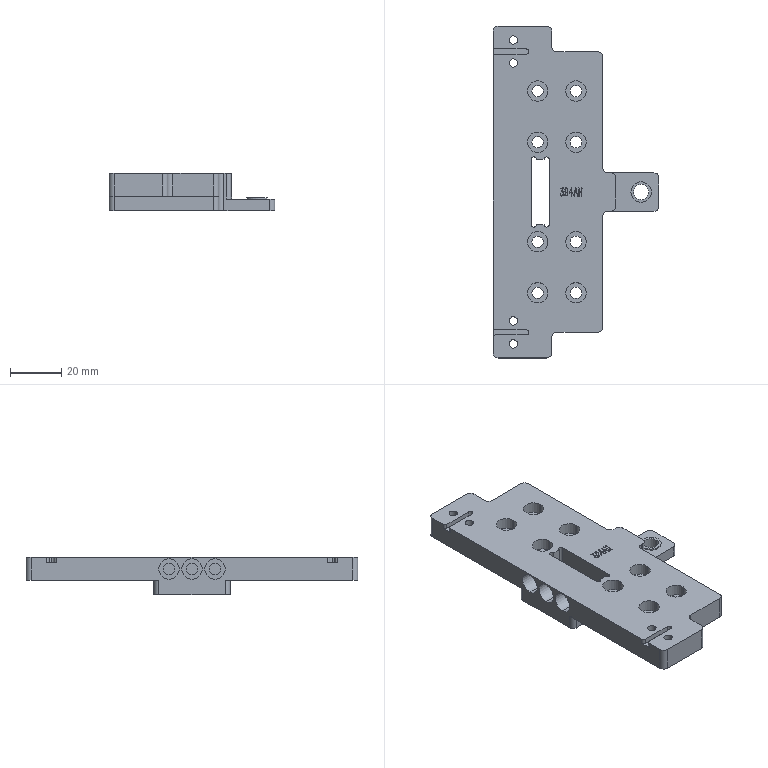NC program | NX | posted with a generic post | part box 65 x 130 x 14.5 mm
Lines 2189 to 4086 of 11202, first 1613 of 1886 lines:
(ZLEVEL_PROFILE_COPY_1_COPY_COPY_1 , TOOL : D10JING)
N4328 T14 M6
N4330 G54
N4332 G17 G0 G90 X64.645 Y-39.348 B0. C0. S9500 M3
N4334 G43 Z30. H14
N4336 Z-13.5
N4338 G94 G1 Z-14.5 F1000.
N4340 X63.866 Y-38.
N4342 G3 X63. Y-37.5 R1.
N4344 G1 X-63. F1200.
N4346 G2 X-70. Y-30.5 R7.
N4348 G1 Y-11.5
N4350 G2 X-63. Y-4.5 R7.
N4352 G1 X-60.
N4354 Y8.5
N4356 G2 X-53. Y15.5 R7.
N4358 G1 X-12.5
N4360 Y30.5
N4362 G2 X-5.5 Y37.5 R7.
N4364 G1 X5.5
N4366 G2 X12.5 Y30.5 R7.
N4368 G1 Y15.5
N4370 X53.
N4372 G2 X60. Y8.5 R7.
N4374 G1 Y-4.5
N4376 X63.
N4378 G2 X70. Y-11.5 R7.
N4380 G1 Y-30.5
N4382 G2 X63. Y-37.5 R7.
N4384 G3 X62.134 Y-38. R1.
N4386 G1 X61.268 Y-39.5
N4388 Z-13.5
N4390 G0 Z30.
N4392 M5
(FLOOR_WALL , TOOL : D4)
N4394 T11 M6
N4396 G54
N4398 G17 G0 G90 X-7.417 Y24.39 B0. C0. S9500 M3
N4400 G43 Z30. H11
N4402 Z-8.
N4404 G94 G1 Z-9.5 F1250.
N4406 X-6.2 Y25.093
N4408 G3 X-6. Y25.44 R0.4
N4410 G1 Y25.56
N4412 G2 X-4.32 Y29.664 R6.
N4414 G1 Y21.336
N4416 G3 X-2.64 Y20.112 R6.
N4418 G1 Y30.888
N4420 G2 X-0.96 Y31.423 R6.
N4422 G1 Y19.577
N4424 G3 X0. Y19.5 R6.
N4426 X0.72 Y19.543 R6.
N4428 G1 X0.719 Y31.457
N4430 G2 X2.399 Y30.999 R6.
N4432 G1 X2.4 Y20.001
N4434 G2 X2.2 Y19.654 R0.4
N4436 G1 X3.742 Y19.
N4438 Z-8.
N4440 G0 Z30.
N4442 X11. Y14.995
N4444 Z-8.5
N4446 G1 Z-10.
N4448 X9.846 Y16.993
N4450 G3 X9.5 Y17.193 R0.4
N4452 G1 X7.5
N4454 G3 X5.5 Y17.7 R4.2
N4456 G1 X-5.5
N4458 G3 X-7.5 Y17.193 R4.2
N4460 G1 X-9.5
N4462 Y19.151
N4464 X9.5
N4466 Y21.109
N4468 X4.378
N4470 G3 X5.703 Y23.068 R6.2
N4472 G1 X9.5
N4474 Y25.026
N4476 X6.182
N4478 G3 X6.02 Y26.984 R6.2
N4480 G1 X9.5
N4482 Y28.942
N4484 X5.157
N4486 G3 X3.046 Y30.9 R6.2
N4488 G1 X9.48
N4490 G2 X9.826 Y30.7 R0.4
N4492 G1 X11. Y28.667
N4494 Z-8.5
N4496 G0 Z30.
N4498 X4.378 Y21.109
N4500 Z-8.5
N4502 G1 Z-10.
N4504 G2 X-4.378 Y21.109 R6.2
N4506 G1 X-9.5
N4508 Y23.068
N4510 X-5.703
N4512 G2 X-6.182 Y25.026 R6.2
N4514 G1 X-9.5
N4516 Y26.984
N4518 X-6.02
N4520 G2 X-5.157 Y28.942 R6.2
N4522 G1 X-9.5
N4524 Y30.5
N4526 G2 X-9.48 Y30.9 R4.
N4528 G1 X-3.046
N4530 Z-8.5
N4532 G0 Z30.
N4534 X10.209 Y33.341
N4536 Z-8.5
N4538 G1 Z-10.
N4540 X9.077 Y32.658
N4542 G3 X8.731 Y32.858 R0.4
N4544 G1 X-8.731
N4546 G3 X-9.077 Y32.658 R0.4
N4548 G1 X-10.209 Y33.341
N4550 Z-8.5
N4552 G0 Z30.
N4554 X-11. Y14.
N4556 Z-8.5
N4558 G1 Z-10.
N4560 X-9.711 Y13.67
N4562 G3 X-9.47 Y13.989 R0.4
N4564 G2 X-5.5 Y17.5 R4.
N4566 G1 X5.5
N4568 G2 X9.47 Y13.989 R4.
N4570 G3 X9.711 Y13.67 R0.4
N4572 G1 X11. Y14.
N4574 Z-8.5
N4576 G0 Z30.
N4578 X-1.744 Y33.
N4580 Z-8.5
N4582 G1 Z-10.
N4584 X-0.346 Y31.7
N4586 G3 X0. Y31.5 R0.4
N4588 G2 X6. Y25.5 R6.
N4590 X0. Y31.5 R-6.
N4592 G3 X0.346 Y31.7 R0.4
N4594 G1 X1.162 Y33.112
N4596 Z-8.5
N4598 G0 Z30.
(HOLE_MILLING , TOOL : D4)
N4600 X0. Y25.5
N4602 Z-9.
N4604 G3 X0.45 Y25.95 R0.45
N4606 X0. Y26.4 R0.45
N4608 X0. Y26.4 Z-9.4 I0. J-0.9
N4610 X0. Y26.4 Z-9.8 I0. J-0.9
N4612 X0. Y26.4 Z-10.2 I0. J-0.9
N4614 X0. Y26.4 Z-10.6 I0. J-0.9
N4616 X0. Y26.4 Z-11. I0. J-0.9
N4618 X0. Y26.4 Z-11.4 I0. J-0.9
N4620 X0. Y26.4 Z-11.8 I0. J-0.9
N4622 X0. Y26.4 Z-12.2 I0. J-0.9
N4624 X0. Y26.4 Z-12.6 I0. J-0.9
N4626 X0. Y26.4 Z-13. I0. J-0.9
N4628 X0. Y26.4 Z-13.4 I0. J-0.9
N4630 X0. Y26.4 Z-13.8 I0. J-0.9
N4632 X0. Y26.4 Z-14.2 I0. J-0.9
N4634 X0.9 Y25.5 Z-14.5 R-0.9
N4636 X0. Y26.4 R0.9
N4638 X0.9 Y25.5 R-0.9
N4640 X0.45 Y25.95 R0.45
N4642 X0. Y25.5 R0.45
N4644 G0 Z30.
(HOLE_MILLING_COPY , TOOL : D4)
N4646 X-39.5 Y0.
N4648 Z0.5
N4650 G3 X-38.5 Y1. R1.
N4652 X-39.5 Y2. R1.
N4654 X-39.5 Y2. Z0.1 I0. J-2.
N4656 X-39.5 Y2. Z-0.3 I0. J-2.
N4658 X-39.5 Y2. Z-0.7 I0. J-2.
N4660 X-39.5 Y2. Z-1.1 I0. J-2.
N4662 X-39.5 Y2. Z-1.5 I0. J-2.
N4664 X-39.5 Y2. Z-1.9 I0. J-2.
N4666 X-39.5 Y2. Z-2.3 I0. J-2.
N4668 X-39.5 Y2. Z-2.7 I0. J-2.
N4670 X-39.5 Y2. Z-3.1 I0. J-2.
N4672 X-39.5 Y2. Z-3.5 I0. J-2.
N4674 X-39.5 Y2. Z-3.9 I0. J-2.
N4676 X-39.5 Y2. Z-4.3 I0. J-2.
N4678 X-37.5 Y0. Z-4.6 R-2.
N4680 X-39.5 Y2. R2.
N4682 X-37.5 Y0. R-2.
N4684 X-38.5 Y1. R1.
N4686 X-39.5 Y0. R1.
N4688 G0 Z30.
N4690 Y-15.
N4692 Z0.5
N4694 G3 X-38.5 Y-14. R1.
N4696 X-39.5 Y-13. R1.
N4698 X-39.5 Y-13. Z0.1 I0. J-2.
N4700 X-39.5 Y-13. Z-0.3 I0. J-2.
N4702 X-39.5 Y-13. Z-0.7 I0. J-2.
N4704 X-39.5 Y-13. Z-1.1 I0. J-2.
N4706 X-39.5 Y-13. Z-1.5 I0. J-2.
N4708 X-39.5 Y-13. Z-1.9 I0. J-2.
N4710 X-39.5 Y-13. Z-2.3 I0. J-2.
N4712 X-39.5 Y-13. Z-2.7 I0. J-2.
N4714 X-39.5 Y-13. Z-3.1 I0. J-2.
N4716 X-39.5 Y-13. Z-3.5 I0. J-2.
N4718 X-39.5 Y-13. Z-3.9 I0. J-2.
N4720 X-39.5 Y-13. Z-4.3 I0. J-2.
N4722 X-37.5 Y-15. Z-4.6 R-2.
N4724 X-39.5 Y-13. R2.
N4726 X-37.5 Y-15. R-2.
N4728 X-38.5 Y-14. R1.
N4730 X-39.5 Y-15. R1.
N4732 G0 Z30.
N4734 X-19.5
N4736 Z0.5
N4738 G3 X-18.5 Y-14. R1.
N4740 X-19.5 Y-13. R1.
N4742 X-19.5 Y-13. Z0.1 I0. J-2.
N4744 X-19.5 Y-13. Z-0.3 I0. J-2.
N4746 X-19.5 Y-13. Z-0.7 I0. J-2.
N4748 X-19.5 Y-13. Z-1.1 I0. J-2.
N4750 X-19.5 Y-13. Z-1.5 I0. J-2.
N4752 X-19.5 Y-13. Z-1.9 I0. J-2.
N4754 X-19.5 Y-13. Z-2.3 I0. J-2.
N4756 X-19.5 Y-13. Z-2.7 I0. J-2.
N4758 X-19.5 Y-13. Z-3.1 I0. J-2.
N4760 X-19.5 Y-13. Z-3.5 I0. J-2.
N4762 X-19.5 Y-13. Z-3.9 I0. J-2.
N4764 X-19.5 Y-13. Z-4.3 I0. J-2.
N4766 X-17.5 Y-15. Z-4.6 R-2.
N4768 X-19.5 Y-13. R2.
N4770 X-17.5 Y-15. R-2.
N4772 X-18.5 Y-14. R1.
N4774 X-19.5 Y-15. R1.
N4776 G0 Z30.
N4778 Y0.
N4780 Z0.5
N4782 G3 X-18.5 Y1. R1.
N4784 X-19.5 Y2. R1.
N4786 X-19.5 Y2. Z0.1 I0. J-2.
N4788 X-19.5 Y2. Z-0.3 I0. J-2.
N4790 X-19.5 Y2. Z-0.7 I0. J-2.
N4792 X-19.5 Y2. Z-1.1 I0. J-2.
N4794 X-19.5 Y2. Z-1.5 I0. J-2.
N4796 X-19.5 Y2. Z-1.9 I0. J-2.
N4798 X-19.5 Y2. Z-2.3 I0. J-2.
N4800 X-19.5 Y2. Z-2.7 I0. J-2.
N4802 X-19.5 Y2. Z-3.1 I0. J-2.
N4804 X-19.5 Y2. Z-3.5 I0. J-2.
N4806 X-19.5 Y2. Z-3.9 I0. J-2.
N4808 X-19.5 Y2. Z-4.3 I0. J-2.
N4810 X-17.5 Y0. Z-4.6 R-2.
N4812 X-19.5 Y2. R2.
N4814 X-17.5 Y0. R-2.
N4816 X-18.5 Y1. R1.
N4818 X-19.5 Y0. R1.
N4820 G0 Z30.
N4822 X19.5
N4824 Z0.5
N4826 G3 X20.5 Y1. R1.
N4828 X19.5 Y2. R1.
N4830 X19.5 Y2. Z0.1 I0. J-2.
N4832 X19.5 Y2. Z-0.3 I0. J-2.
N4834 X19.5 Y2. Z-0.7 I0. J-2.
N4836 X19.5 Y2. Z-1.1 I0. J-2.
N4838 X19.5 Y2. Z-1.5 I0. J-2.
N4840 X19.5 Y2. Z-1.9 I0. J-2.
N4842 X19.5 Y2. Z-2.3 I0. J-2.
N4844 X19.5 Y2. Z-2.7 I0. J-2.
N4846 X19.5 Y2. Z-3.1 I0. J-2.
N4848 X19.5 Y2. Z-3.5 I0. J-2.
N4850 X19.5 Y2. Z-3.9 I0. J-2.
N4852 X19.5 Y2. Z-4.3 I0. J-2.
N4854 X21.5 Y0. Z-4.6 R-2.
N4856 X19.5 Y2. R2.
N4858 X21.5 Y0. R-2.
N4860 X20.5 Y1. R1.
N4862 X19.5 Y0. R1.
N4864 G0 Z30.
N4866 Y-15.
N4868 Z0.5
N4870 G3 X20.5 Y-14. R1.
N4872 X19.5 Y-13. R1.
N4874 X19.5 Y-13. Z0.1 I0. J-2.
N4876 X19.5 Y-13. Z-0.3 I0. J-2.
N4878 X19.5 Y-13. Z-0.7 I0. J-2.
N4880 X19.5 Y-13. Z-1.1 I0. J-2.
N4882 X19.5 Y-13. Z-1.5 I0. J-2.
N4884 X19.5 Y-13. Z-1.9 I0. J-2.
N4886 X19.5 Y-13. Z-2.3 I0. J-2.
N4888 X19.5 Y-13. Z-2.7 I0. J-2.
N4890 X19.5 Y-13. Z-3.1 I0. J-2.
N4892 X19.5 Y-13. Z-3.5 I0. J-2.
N4894 X19.5 Y-13. Z-3.9 I0. J-2.
N4896 X19.5 Y-13. Z-4.3 I0. J-2.
N4898 X21.5 Y-15. Z-4.6 R-2.
N4900 X19.5 Y-13. R2.
N4902 X21.5 Y-15. R-2.
N4904 X20.5 Y-14. R1.
N4906 X19.5 Y-15. R1.
N4908 G0 Z30.
N4910 X39.5
N4912 Z0.5
N4914 G3 X40.5 Y-14. R1.
N4916 X39.5 Y-13. R1.
N4918 X39.5 Y-13. Z0.1 I0. J-2.
N4920 X39.5 Y-13. Z-0.3 I0. J-2.
N4922 X39.5 Y-13. Z-0.7 I0. J-2.
N4924 X39.5 Y-13. Z-1.1 I0. J-2.
N4926 X39.5 Y-13. Z-1.5 I0. J-2.
N4928 X39.5 Y-13. Z-1.9 I0. J-2.
N4930 X39.5 Y-13. Z-2.3 I0. J-2.
N4932 X39.5 Y-13. Z-2.7 I0. J-2.
N4934 X39.5 Y-13. Z-3.1 I0. J-2.
N4936 X39.5 Y-13. Z-3.5 I0. J-2.
N4938 X39.5 Y-13. Z-3.9 I0. J-2.
N4940 X39.5 Y-13. Z-4.3 I0. J-2.
N4942 X41.5 Y-15. Z-4.6 R-2.
N4944 X39.5 Y-13. R2.
N4946 X41.5 Y-15. R-2.
N4948 X40.5 Y-14. R1.
N4950 X39.5 Y-15. R1.
N4952 G0 Z30.
N4954 Y0.
N4956 Z0.5
N4958 G3 X40.5 Y1. R1.
N4960 X39.5 Y2. R1.
N4962 X39.5 Y2. Z0.1 I0. J-2.
N4964 X39.5 Y2. Z-0.3 I0. J-2.
N4966 X39.5 Y2. Z-0.7 I0. J-2.
N4968 X39.5 Y2. Z-1.1 I0. J-2.
N4970 X39.5 Y2. Z-1.5 I0. J-2.
N4972 X39.5 Y2. Z-1.9 I0. J-2.
N4974 X39.5 Y2. Z-2.3 I0. J-2.
N4976 X39.5 Y2. Z-2.7 I0. J-2.
N4978 X39.5 Y2. Z-3.1 I0. J-2.
N4980 X39.5 Y2. Z-3.5 I0. J-2.
N4982 X39.5 Y2. Z-3.9 I0. J-2.
N4984 X39.5 Y2. Z-4.3 I0. J-2.
N4986 X41.5 Y0. Z-4.6 R-2.
N4988 X39.5 Y2. R2.
N4990 X41.5 Y0. R-2.
N4992 X40.5 Y1. R1.
N4994 X39.5 Y0. R1.
N4996 G0 Z30.
(ZLEVEL_PROFILE , TOOL : D4)
N4998 X1.453 Y-15.4
N5000 Z1.5
N5002 G1 X10.65 Z1.018 F1000.
N5004 Y-12.6 Z0.871
N5006 X-10.653 Z-0.245
N5008 X-10.65 Y-12.637 Z-0.247
N5010 Y-15.363 Z-0.39
N5012 X-10.653 Y-15.4 Z-0.392
N5014 X10.65 F1800.
N5016 Y-12.6
N5018 X-10.653
N5020 X-10.65 Y-12.637
N5022 Y-15.363
N5024 X-10.653 Y-15.4
N5026 X-10.508 Z-0.394
N5028 X10.64 Z-0.764
N5030 X10.65 Y-15.265 Z-0.766
N5032 Y-14.251 Z-0.784
N5034 Y-12.6
N5036 X-10.653
N5038 X-10.65 Y-12.637
N5040 Y-15.363
N5042 X-10.653 Y-15.4
N5044 X-10.508 Z-0.786
N5046 X10.64 Z-1.155
N5048 X10.65 Y-15.265 Z-1.158
N5050 Y-14.251 Z-1.176
N5052 Y-12.6
N5054 X-10.653
N5056 X-10.65 Y-12.637
N5058 Y-15.363
N5060 X-10.653 Y-15.4
N5062 X-10.508 Z-1.178
N5064 X10.64 Z-1.547
N5066 X10.65 Y-15.265 Z-1.55
N5068 Y-14.251 Z-1.568
N5070 Y-12.6
N5072 X-10.653
N5074 X-10.65 Y-12.637
N5076 Y-15.363
N5078 X-10.653 Y-15.4
N5080 X-10.508 Z-1.57
N5082 X10.64 Z-1.939
N5084 X10.65 Y-15.265 Z-1.942
N5086 Y-14.251 Z-1.959
N5088 Y-12.6
N5090 X-10.653
N5092 X-10.65 Y-12.637
N5094 Y-15.363
N5096 X-10.653 Y-15.4
N5098 X-10.508 Z-1.962
N5100 X10.64 Z-2.331
N5102 X10.65 Y-15.265 Z-2.334
N5104 Y-14.251 Z-2.351
N5106 Y-12.6
N5108 X-10.653
N5110 X-10.65 Y-12.637
N5112 Y-15.363
N5114 X-10.653 Y-15.4
N5116 X-10.508 Z-2.354
N5118 X10.64 Z-2.723
N5120 X10.65 Y-15.265 Z-2.726
N5122 Y-14.251 Z-2.743
N5124 Y-12.6
N5126 X-10.653
N5128 X-10.65 Y-12.637
N5130 Y-15.363
N5132 X-10.653 Y-15.4
N5134 X-10.508 Z-2.746
N5136 X10.64 Z-3.115
N5138 X10.65 Y-15.265 Z-3.117
N5140 Y-14.251 Z-3.135
N5142 Y-12.6
N5144 X-10.653
N5146 X-10.65 Y-12.637
N5148 Y-15.363
N5150 X-10.653 Y-15.4
N5152 X-10.508 Z-3.138
N5154 X10.64 Z-3.507
N5156 X10.65 Y-15.265 Z-3.509
N5158 Y-14.251 Z-3.527
N5160 Y-12.6
N5162 X-10.652
N5164 X-10.65 Y-12.637
N5166 Y-15.363
N5168 X-10.652 Y-15.4
N5170 X-10.508 Z-3.53
N5172 X10.64 Z-3.899
N5174 X10.65 Y-15.265 Z-3.901
N5176 Y-14.251 Z-3.919
N5178 Y-12.6
N5180 X-10.652
N5182 X-10.65 Y-12.637
N5184 Y-15.363
N5186 X-10.652 Y-15.4
N5188 X-10.508 Z-3.921
N5190 X10.64 Z-4.291
N5192 X10.65 Y-15.265 Z-4.293
N5194 Y-14.251 Z-4.311
N5196 Y-12.6
N5198 X-10.652
N5200 X-10.65 Y-12.637
N5202 Y-15.363
N5204 X-10.652 Y-15.4
N5206 X-10.508 Z-4.313
N5208 X10.64 Z-4.682
N5210 X10.65 Y-15.265 Z-4.685
N5212 Y-14.251 Z-4.703
N5214 Y-12.6
N5216 X-10.652
N5218 X-10.65 Y-12.637
N5220 Y-15.363
N5222 X-10.652 Y-15.4
N5224 X-10.508 Z-4.705
N5226 X10.64 Z-5.074
N5228 X10.65 Y-15.265 Z-5.077
N5230 Y-14.251 Z-5.095
N5232 Y-12.6
N5234 X-10.652
N5236 X-10.65 Y-12.637
N5238 Y-15.363
N5240 X-10.652 Y-15.4
N5242 X-10.508 Z-5.097
N5244 X10.64 Z-5.466
N5246 X10.65 Y-15.265 Z-5.469
N5248 Y-14.251 Z-5.486
N5250 Y-12.6
N5252 X-10.652
N5254 X-10.65 Y-12.637
N5256 Y-15.363
N5258 X-10.652 Y-15.4
N5260 X-10.508 Z-5.489
N5262 X10.64 Z-5.858
N5264 X10.65 Y-15.265 Z-5.861
N5266 Y-14.251 Z-5.878
N5268 Y-12.6
N5270 X-10.652
N5272 X-10.65 Y-12.637
N5274 Y-15.363
N5276 X-10.652 Y-15.4
N5278 X-10.508 Z-5.881
N5280 X10.64 Z-6.25
N5282 X10.65 Y-15.265 Z-6.253
N5284 Y-14.251 Z-6.27
N5286 Y-12.6
N5288 X-10.652
N5290 X-10.65 Y-12.637
N5292 Y-15.363
N5294 X-10.652 Y-15.4
N5296 X-10.508 Z-6.273
N5298 X10.64 Z-6.642
N5300 X10.65 Y-15.265 Z-6.644
N5302 Y-14.251 Z-6.662
N5304 Y-12.6
N5306 X-10.652
N5308 X-10.65 Y-12.637
N5310 Y-15.363
N5312 X-10.652 Y-15.4
N5314 X-10.508 Z-6.665
N5316 X10.64 Z-7.034
N5318 X10.65 Y-15.265 Z-7.036
N5320 Y-14.251 Z-7.054
N5322 Y-12.6
N5324 X-10.652
N5326 X-10.65 Y-12.637
N5328 Y-15.363
N5330 X-10.652 Y-15.4
N5332 X-10.508 Z-7.057
N5334 X10.64 Z-7.426
N5336 X10.65 Y-15.265 Z-7.428
N5338 Y-14.251 Z-7.446
N5340 Y-12.6
N5342 X-10.652
N5344 X-10.65 Y-12.637
N5346 Y-15.363
N5348 X-10.652 Y-15.4
N5350 X-10.508 Z-7.448
N5352 X10.64 Z-7.818
N5354 X10.65 Y-15.265 Z-7.82
N5356 Y-14.251 Z-7.838
N5358 Y-12.6
N5360 X-10.652
N5362 X-10.65 Y-12.637
N5364 Y-15.363
N5366 X-10.652 Y-15.4
N5368 X-10.508 Z-7.84
N5370 X10.64 Z-8.21
N5372 X10.65 Y-15.265 Z-8.212
N5374 Y-14.251 Z-8.23
N5376 Y-12.6
N5378 X-10.652
N5380 X-10.65 Y-12.637
N5382 Y-15.363
N5384 X-10.652 Y-15.4
N5386 X-10.508 Z-8.232
N5388 X10.64 Z-8.601
N5390 X10.65 Y-15.265 Z-8.604
N5392 Y-14.251 Z-8.622
N5394 Y-12.6
N5396 X-10.652
N5398 X-10.65 Y-12.637
N5400 Y-15.363
N5402 X-10.652 Y-15.4
N5404 X-10.508 Z-8.624
N5406 X10.64 Z-8.993
N5408 X10.65 Y-15.265 Z-8.996
N5410 Y-14.251 Z-9.014
N5412 Y-12.6
N5414 X-10.652
N5416 X-10.65 Y-12.637
N5418 Y-15.363
N5420 X-10.652 Y-15.4
N5422 X-10.508 Z-9.016
N5424 X10.64 Z-9.385
N5426 X10.65 Y-15.265 Z-9.388
N5428 Y-14.251 Z-9.405
N5430 Y-12.6
N5432 X-10.652
N5434 X-10.65 Y-12.637
N5436 Y-15.363
N5438 X-10.652 Y-15.4
N5440 X-10.508 Z-9.408
N5442 X10.64 Z-9.777
N5444 X10.65 Y-15.265 Z-9.78
N5446 Y-14.251 Z-9.797
N5448 Y-12.6
N5450 X-10.652
N5452 X-10.65 Y-12.637
N5454 Y-15.363
N5456 X-10.652 Y-15.4
N5458 X-10.508 Z-9.8
N5460 X10.64 Z-10.169
N5462 X10.65 Y-15.265 Z-10.171
N5464 Y-14.251 Z-10.189
N5466 Y-12.6
N5468 X-10.652
N5470 X-10.65 Y-12.637
N5472 Y-15.363
N5474 X-10.652 Y-15.4
N5476 X-10.508 Z-10.192
N5478 X10.64 Z-10.561
N5480 X10.65 Y-15.265 Z-10.563
N5482 Y-14.251 Z-10.581
N5484 Y-12.6
N5486 X-10.652
N5488 X-10.65 Y-12.637
N5490 Y-15.363
N5492 X-10.652 Y-15.4
N5494 X-10.508 Z-10.584
N5496 X10.64 Z-10.953
N5498 X10.65 Y-15.265 Z-10.955
N5500 Y-14.251 Z-10.973
N5502 Y-12.6
N5504 X-10.652
N5506 X-10.65 Y-12.637
N5508 Y-15.363
N5510 X-10.652 Y-15.4
N5512 X-10.508 Z-10.976
N5514 X10.64 Z-11.345
N5516 X10.65 Y-15.265 Z-11.347
N5518 Y-14.251 Z-11.365
N5520 Y-12.6
N5522 X-10.652
N5524 X-10.65 Y-12.637
N5526 Y-15.363
N5528 X-10.652 Y-15.4
N5530 X-10.508 Z-11.367
N5532 X10.64 Z-11.737
N5534 X10.65 Y-15.265 Z-11.739
N5536 Y-14.251 Z-11.757
N5538 Y-12.6
N5540 X-10.652
N5542 X-10.65 Y-12.637
N5544 Y-15.363
N5546 X-10.652 Y-15.4
N5548 X-10.508 Z-11.759
N5550 X10.64 Z-12.128
N5552 X10.65 Y-15.265 Z-12.131
N5554 Y-14.251 Z-12.149
N5556 Y-12.6
N5558 X-10.652
N5560 X-10.65 Y-12.637
N5562 Y-15.363
N5564 X-10.652 Y-15.4
N5566 X-10.508 Z-12.151
N5568 X10.64 Z-12.52
N5570 X10.65 Y-15.265 Z-12.523
N5572 Y-14.251 Z-12.541
N5574 Y-12.6
N5576 X-10.652
N5578 X-10.65 Y-12.637
N5580 Y-15.363
N5582 X-10.652 Y-15.4
N5584 X-10.508 Z-12.543
N5586 X10.64 Z-12.912
N5588 X10.65 Y-15.265 Z-12.915
N5590 Y-14.251 Z-12.932
N5592 Y-12.6
N5594 X-10.652
N5596 X-10.65 Y-12.637
N5598 Y-15.363
N5600 X-10.652 Y-15.4
N5602 X-10.508 Z-12.935
N5604 X10.64 Z-13.304
N5606 X10.65 Y-15.265 Z-13.307
N5608 Y-14.251 Z-13.324
N5610 Y-12.6
N5612 X-10.652
N5614 X-10.65 Y-12.637
N5616 Y-15.363
N5618 X-10.652 Y-15.4
N5620 X-10.508 Z-13.327
N5622 X10.64 Z-13.696
N5624 X10.65 Y-15.265 Z-13.699
N5626 Y-14.251 Z-13.716
N5628 Y-12.6
N5630 X-10.652
N5632 X-10.65 Y-12.637
N5634 Y-15.363
N5636 X-10.652 Y-15.4
N5638 X-10.508 Z-13.719
N5640 X10.64 Z-14.088
N5642 X10.65 Y-15.265 Z-14.09
N5644 Y-14.251 Z-14.108
N5646 Y-12.6
N5648 X-10.652
N5650 X-10.65 Y-12.637
N5652 Y-15.363
N5654 X-10.652 Y-15.4
N5656 X-10.508 Z-14.111
N5658 X10.64 Z-14.48
N5660 X10.65 Y-15.265 Z-14.482
N5662 Y-14.251 Z-14.5
N5664 Y-12.6
N5666 X-10.652
N5668 X-10.65 Y-12.637
N5670 Y-15.363
N5672 X-10.652 Y-15.4
N5674 X10.65
N5676 Y-14.251
N5678 Z-13.
N5680 G0 Z30.
(ZLEVEL_PROFILE_COPY , TOOL : D4)
N5682 X-60.846 Y-6.7
N5684 Z-0.392
N5686 G1 X-60.499 Y-7.3 F1000.
N5688 G3 X-60.153 Y-7.5 R0.4
N5690 G1 X-57.06 F1800.
N5692 X-56.998 Y-7.502
N5694 X-57. Y-7.486
N5696 Y-4.347
N5698 G3 X-57.2 Y-4.001 R0.4
N5700 G1 X-57.8 Y-3.654
N5702 G0 X-60.846 Y-6.7 Z-0.784
N5704 G1 X-60.499 Y-7.3 F1000.
N5706 G3 X-60.153 Y-7.5 R0.4
N5708 G1 X-57.06 F1800.
N5710 X-56.998 Y-7.502
N5712 X-57. Y-7.486
N5714 Y-4.347
N5716 G3 X-57.2 Y-4.001 R0.4
N5718 G1 X-57.8 Y-3.654
N5720 G0 X-60.846 Y-6.7 Z-1.176
N5722 G1 X-60.499 Y-7.3 F1000.
N5724 G3 X-60.153 Y-7.5 R0.4
N5726 G1 X-57.06 F1800.
N5728 X-56.998 Y-7.502
N5730 X-57. Y-7.486
N5732 Y-4.347
N5734 G3 X-57.2 Y-4.001 R0.4
N5736 G1 X-57.8 Y-3.654
N5738 G0 X-60.846 Y-6.7 Z-1.568
N5740 G1 X-60.499 Y-7.3 F1000.
N5742 G3 X-60.153 Y-7.5 R0.4
N5744 G1 X-57.06 F1800.
N5746 X-56.998 Y-7.502
N5748 X-57. Y-7.486
N5750 Y-4.347
N5752 G3 X-57.2 Y-4.001 R0.4
N5754 G1 X-57.8 Y-3.654
N5756 G0 X-60.846 Y-6.7 Z-1.959
N5758 G1 X-60.499 Y-7.3 F1000.
N5760 G3 X-60.153 Y-7.5 R0.4
N5762 G1 X-57.06 F1800.
N5764 X-56.998 Y-7.502
N5766 X-57. Y-7.486
N5768 Y-4.347
N5770 G3 X-57.2 Y-4.001 R0.4
N5772 G1 X-57.8 Y-3.654
N5774 G0 X-60.846 Y-6.7 Z-2.351
N5776 G1 X-60.499 Y-7.3 F1000.
N5778 G3 X-60.153 Y-7.5 R0.4
N5780 G1 X-57.06 F1800.
N5782 X-56.998 Y-7.502
N5784 X-57. Y-7.486
N5786 Y-4.347
N5788 G3 X-57.2 Y-4.001 R0.4
N5790 G1 X-57.8 Y-3.654
N5792 G0 X-60.846 Y-6.7 Z-2.743
N5794 G1 X-60.499 Y-7.3 F1000.
N5796 G3 X-60.153 Y-7.5 R0.4
N5798 G1 X-57.06 F1800.
N5800 X-56.998 Y-7.502
N5802 X-57. Y-7.486
N5804 Y-4.347
N5806 G3 X-57.2 Y-4.001 R0.4
N5808 G1 X-57.8 Y-3.654
N5810 G0 X-60.846 Y-6.7 Z-3.135
N5812 G1 X-60.499 Y-7.3 F1000.
N5814 G3 X-60.153 Y-7.5 R0.4
N5816 G1 X-57.06 F1800.
N5818 X-56.998 Y-7.502
N5820 X-57. Y-7.486
N5822 Y-4.347
N5824 G3 X-57.2 Y-4.001 R0.4
N5826 G1 X-57.8 Y-3.654
N5828 G0 X-60.846 Y-6.7 Z-3.527
N5830 G1 X-60.499 Y-7.3 F1000.
N5832 G3 X-60.153 Y-7.5 R0.4
N5834 G1 X-57.06 F1800.
N5836 X-56.998 Y-7.502
N5838 X-57. Y-7.486
N5840 Y-4.347
N5842 G3 X-57.2 Y-4.001 R0.4
N5844 G1 X-57.8 Y-3.654
N5846 G0 X-60.846 Y-6.7 Z-3.919
N5848 G1 X-60.499 Y-7.3 F1000.
N5850 G3 X-60.153 Y-7.5 R0.4
N5852 G1 X-57.06 F1800.
N5854 X-56.999 Y-7.501
N5856 X-57. Y-7.486
N5858 Y-4.347
N5860 G3 X-57.2 Y-4.001 R0.4
N5862 G1 X-57.8 Y-3.654
N5864 G0 X-60.846 Y-6.7 Z-4.311
N5866 G1 X-60.499 Y-7.3 F1000.
N5868 G3 X-60.153 Y-7.5 R0.4
N5870 G1 X-57.06 F1800.
N5872 X-56.999 Y-7.501
N5874 X-57. Y-7.486
N5876 Y-4.347
N5878 G3 X-57.2 Y-4.001 R0.4
N5880 G1 X-57.8 Y-3.654
N5882 G0 X-60.846 Y-6.7 Z-4.703
N5884 G1 X-60.499 Y-7.3 F1000.
N5886 G3 X-60.153 Y-7.5 R0.4
N5888 G1 X-57.06 F1800.
N5890 X-56.999 Y-7.501
N5892 X-57. Y-7.486
N5894 Y-4.347
N5896 G3 X-57.2 Y-4.001 R0.4
N5898 G1 X-57.8 Y-3.654
N5900 G0 X-60.846 Y-6.7 Z-5.095
N5902 G1 X-60.499 Y-7.3 F1000.
N5904 G3 X-60.153 Y-7.5 R0.4
N5906 G1 X-57.06 F1800.
N5908 X-56.999 Y-7.501
N5910 X-57. Y-7.486
N5912 Y-4.347
N5914 G3 X-57.2 Y-4.001 R0.4
N5916 G1 X-57.8 Y-3.654
N5918 G0 X-60.846 Y-6.7 Z-5.486
N5920 G1 X-60.499 Y-7.3 F1000.
N5922 G3 X-60.153 Y-7.5 R0.4
N5924 G1 X-57.06 F1800.
N5926 X-56.999 Y-7.501
N5928 X-57. Y-4.347
N5930 G3 X-57.2 Y-4.001 R0.4
N5932 G1 X-57.8 Y-3.654
N5934 G0 X-60.846 Y-6.7 Z-5.878
N5936 G1 X-60.499 Y-7.3 F1000.
N5938 G3 X-60.153 Y-7.5 R0.4
N5940 G1 X-57.06 F1800.
N5942 X-56.999 Y-7.501
N5944 X-57. Y-4.347
N5946 G3 X-57.2 Y-4.001 R0.4
N5948 G1 X-57.8 Y-3.654
N5950 G0 X-60.846 Y-6.7 Z-6.27
N5952 G1 X-60.499 Y-7.3 F1000.
N5954 G3 X-60.153 Y-7.5 R0.4
N5956 G1 X-57.06 F1800.
N5958 X-56.999 Y-7.501
N5960 X-57. Y-4.347
N5962 G3 X-57.2 Y-4.001 R0.4
N5964 G1 X-57.8 Y-3.654
N5966 G0 X-60.846 Y-6.7 Z-6.662
N5968 G1 X-60.499 Y-7.3 F1000.
N5970 G3 X-60.153 Y-7.5 R0.4
N5972 G1 X-57.06 F1800.
N5974 X-56.999 Y-7.501
N5976 X-57. Y-4.347
N5978 G3 X-57.2 Y-4.001 R0.4
N5980 G1 X-57.8 Y-3.654
N5982 G0 X-60.846 Y-6.7 Z-7.054
N5984 G1 X-60.499 Y-7.3 F1000.
N5986 G3 X-60.153 Y-7.5 R0.4
N5988 G1 X-57.06 F1800.
N5990 X-57.
N5992 Y-4.347
N5994 G3 X-57.2 Y-4.001 R0.4
N5996 G1 X-57.8 Y-3.654
N5998 G0 X-60.846 Y-6.7 Z-7.446
N6000 G1 X-60.499 Y-7.3 F1000.
N6002 G3 X-60.153 Y-7.5 R0.4
N6004 G1 X-57.06 F1800.
N6006 X-57.
N6008 Y-4.347
N6010 G3 X-57.2 Y-4.001 R0.4
N6012 G1 X-57.8 Y-3.654
N6014 G0 X-60.846 Y-6.7 Z-7.838
N6016 G1 X-60.499 Y-7.3 F1000.
N6018 G3 X-60.153 Y-7.5 R0.4
N6020 G1 X-57.06 F1800.
N6022 X-57.
N6024 Y-4.347
N6026 G3 X-57.2 Y-4.001 R0.4
N6028 G1 X-57.8 Y-3.654
N6030 G0 X-60.846 Y-6.7 Z-8.23
N6032 G1 X-60.499 Y-7.3 F1000.
N6034 G3 X-60.153 Y-7.5 R0.4
N6036 G1 X-57.06 F1800.
N6038 X-57.
N6040 Y-4.347
N6042 G3 X-57.2 Y-4.001 R0.4
N6044 G1 X-57.8 Y-3.654
N6046 G0 X-60.846 Y-6.7 Z-8.622
N6048 G1 X-60.499 Y-7.3 F1000.
N6050 G3 X-60.153 Y-7.5 R0.4
N6052 G1 X-57.06 F1800.
N6054 X-57.
N6056 Y-4.347
N6058 G3 X-57.2 Y-4.001 R0.4
N6060 G1 X-57.8 Y-3.654
N6062 G0 X-60.846 Y-6.7 Z-9.014
N6064 G1 X-60.499 Y-7.3 F1000.
N6066 G3 X-60.153 Y-7.5 R0.4
N6068 G1 X-57. F1800.
N6070 Y-4.347
N6072 G3 X-57.2 Y-4.001 R0.4
N6074 G1 X-57.8 Y-3.654
N6076 G0 X-60.846 Y-6.7 Z-9.405
N6078 G1 X-60.499 Y-7.3 F1000.
N6080 G3 X-60.153 Y-7.5 R0.4
N6082 G1 X-57. F1800.
N6084 Y-4.347
N6086 G3 X-57.2 Y-4.001 R0.4
N6088 G1 X-57.8 Y-3.654
N6090 G0 X-60.846 Y-6.7 Z-9.797
N6092 G1 X-60.499 Y-7.3 F1000.
N6094 G3 X-60.153 Y-7.5 R0.4
N6096 G1 X-57. F1800.
N6098 Y-4.347
N6100 G3 X-57.2 Y-4.001 R0.4
N6102 G1 X-57.8 Y-3.654
N6104 G0 X-60.846 Y-6.7 Z-10.189
N6106 G1 X-60.499 Y-7.3 F1000.
N6108 G3 X-60.153 Y-7.5 R0.4
N6110 G1 X-57. F1800.
N6112 Y-4.347
N6114 G3 X-57.2 Y-4.001 R0.4
N6116 G1 X-57.8 Y-3.654
N6118 G0 X-60.846 Y-6.7 Z-10.581
N6120 G1 X-60.499 Y-7.3 F1000.
N6122 G3 X-60.153 Y-7.5 R0.4
N6124 G1 X-57. F1800.
N6126 Y-4.347
N6128 G3 X-57.2 Y-4.001 R0.4
N6130 G1 X-57.8 Y-3.654
N6132 G0 X-60.846 Y-6.7 Z-10.973
N6134 G1 X-60.499 Y-7.3 F1000.
N6136 G3 X-60.153 Y-7.5 R0.4
N6138 G1 X-57. F1800.
N6140 Y-4.347
N6142 G3 X-57.2 Y-4.001 R0.4
N6144 G1 X-57.8 Y-3.654
N6146 G0 X-60.846 Y-6.7 Z-11.365
N6148 G1 X-60.499 Y-7.3 F1000.
N6150 G3 X-60.153 Y-7.5 R0.4
N6152 G1 X-57. F1800.
N6154 Y-4.347
N6156 G3 X-57.2 Y-4.001 R0.4
N6158 G1 X-57.8 Y-3.654
N6160 G0 X-60.846 Y-6.7 Z-11.757
N6162 G1 X-60.499 Y-7.3 F1000.
N6164 G3 X-60.153 Y-7.5 R0.4
N6166 G1 X-57. F1800.
N6168 Y-4.347
N6170 G3 X-57.2 Y-4.001 R0.4
N6172 G1 X-57.8 Y-3.654
N6174 G0 X-60.846 Y-6.7 Z-12.149
N6176 G1 X-60.499 Y-7.3 F1000.
N6178 G3 X-60.153 Y-7.5 R0.4
N6180 G1 X-57. F1800.
N6182 Y-4.347
N6184 G3 X-57.2 Y-4.001 R0.4
N6186 G1 X-57.8 Y-3.654
N6188 G0 X-60.846 Y-6.7 Z-12.541
N6190 G1 X-60.499 Y-7.3 F1000.
N6192 G3 X-60.153 Y-7.5 R0.4
N6194 G1 X-57. F1800.
N6196 Y-4.347
N6198 G3 X-57.2 Y-4.001 R0.4
N6200 G1 X-57.8 Y-3.654
N6202 G0 X-60.846 Y-6.7 Z-12.932
N6204 G1 X-60.499 Y-7.3 F1000.
N6206 G3 X-60.153 Y-7.5 R0.4
N6208 G1 X-57. F1800.
N6210 Y-4.347
N6212 G3 X-57.2 Y-4.001 R0.4
N6214 G1 X-57.8 Y-3.654
N6216 G0 X-60.846 Y-6.7 Z-13.324
N6218 G1 X-60.499 Y-7.3 F1000.
N6220 G3 X-60.153 Y-7.5 R0.4
N6222 G1 X-57. F1800.
N6224 Y-4.347
N6226 G3 X-57.2 Y-4.001 R0.4
N6228 G1 X-57.8 Y-3.654
N6230 G0 X-60.846 Y-6.7 Z-13.716
N6232 G1 X-60.499 Y-7.3 F1000.
N6234 G3 X-60.153 Y-7.5 R0.4
N6236 G1 X-57. F1800.
N6238 Y-4.347
N6240 G3 X-57.2 Y-4.001 R0.4
N6242 G1 X-57.8 Y-3.654
N6244 G0 X-60.846 Y-6.7 Z-14.108
N6246 G1 X-60.499 Y-7.3 F1000.
N6248 G3 X-60.153 Y-7.5 R0.4
N6250 G1 X-57. F1800.
N6252 Y-4.347
N6254 G3 X-57.2 Y-4.001 R0.4
N6256 G1 X-57.8 Y-3.654
N6258 G0 X-60.846 Y-6.7 Z-14.5
N6260 G1 X-60.499 Y-7.3 F1000.
N6262 G3 X-60.153 Y-7.5 R0.4
N6264 G1 X-57. F1800.
N6266 Y-4.347
N6268 G3 X-57.2 Y-4.001 R0.4
N6270 G1 X-57.8 Y-3.654
N6272 G0 Z30.
N6274 X-13.054 Y13.3
N6276 Z-0.392
N6278 G1 X-12.708 Y12.7 F1000.
N6280 G3 X-12.361 Y12.5 R0.4
N6282 G1 X-9.563 F1800.
N6284 X-9.498 Y12.498
N6286 X-9.5 Y12.514
N6288 Y13.5
N6290 G2 X-9.259 Y14.869 R4.
N6292 G3 X-9.328 Y15.263 R0.4
N6294 G1 X-9.739 Y15.752
N6296 G0 X-13.054 Y13.3 Z-0.784
N6298 G1 X-12.708 Y12.7 F1000.
N6300 G3 X-12.361 Y12.5 R0.4
N6302 G1 X-9.563 F1800.
N6304 X-9.498 Y12.498
N6306 X-9.5 Y12.514
N6308 Y13.5
N6310 G2 X-9.259 Y14.869 R4.
N6312 G3 X-9.328 Y15.263 R0.4
N6314 G1 X-9.739 Y15.752
N6316 G0 X-13.054 Y13.3 Z-1.176
N6318 G1 X-12.708 Y12.7 F1000.
N6320 G3 X-12.361 Y12.5 R0.4
N6322 G1 X-9.563 F1800.
N6324 X-9.498 Y12.498
N6326 X-9.5 Y12.514
N6328 Y13.5
N6330 G2 X-9.259 Y14.869 R4.
N6332 G3 X-9.328 Y15.263 R0.4
N6334 G1 X-9.739 Y15.752
N6336 G0 X-13.054 Y13.3 Z-1.568
N6338 G1 X-12.708 Y12.7 F1000.
N6340 G3 X-12.361 Y12.5 R0.4
N6342 G1 X-9.563 F1800.
N6344 X-9.498 Y12.498
N6346 X-9.5 Y12.514
N6348 Y13.5
N6350 G2 X-9.259 Y14.869 R4.
N6352 G3 X-9.328 Y15.263 R0.4
N6354 G1 X-9.739 Y15.752
N6356 G0 X-13.054 Y13.3 Z-1.959
N6358 G1 X-12.708 Y12.7 F1000.
N6360 G3 X-12.361 Y12.5 R0.4
N6362 G1 X-9.563 F1800.
N6364 X-9.498 Y12.498
N6366 X-9.5 Y12.514
N6368 Y13.5
N6370 G2 X-9.259 Y14.869 R4.
N6372 G3 X-9.328 Y15.263 R0.4
N6374 G1 X-9.739 Y15.752
N6376 G0 X-13.054 Y13.3 Z-2.351
N6378 G1 X-12.708 Y12.7 F1000.
N6380 G3 X-12.361 Y12.5 R0.4
N6382 G1 X-9.563 F1800.
N6384 X-9.498 Y12.498
N6386 X-9.5 Y12.514
N6388 Y13.5
N6390 G2 X-9.259 Y14.869 R4.
N6392 G3 X-9.328 Y15.263 R0.4
N6394 G1 X-9.739 Y15.752
N6396 G0 X-13.054 Y13.3 Z-2.743
N6398 G1 X-12.708 Y12.7 F1000.
N6400 G3 X-12.361 Y12.5 R0.4
N6402 G1 X-9.563 F1800.
N6404 X-9.498 Y12.498
N6406 X-9.5 Y12.514
N6408 Y13.5
N6410 G2 X-9.259 Y14.869 R4.
N6412 G3 X-9.328 Y15.263 R0.4
N6414 G1 X-9.739 Y15.752
N6416 G0 X-13.054 Y13.3 Z-3.135
N6418 G1 X-12.708 Y12.7 F1000.
N6420 G3 X-12.361 Y12.5 R0.4
N6422 G1 X-9.563 F1800.
N6424 X-9.499 Y12.499
N6426 X-9.5 Y12.514
N6428 Y13.5
N6430 G2 X-9.259 Y14.869 R4.
N6432 G3 X-9.328 Y15.263 R0.4
N6434 G1 X-9.739 Y15.752
N6436 G0 X-13.054 Y13.3 Z-3.527
N6438 G1 X-12.708 Y12.7 F1000.
N6440 G3 X-12.361 Y12.5 R0.4
N6442 G1 X-9.563 F1800.
N6444 X-9.499 Y12.499
N6446 X-9.5 Y12.514
N6448 Y13.5
N6450 G2 X-9.259 Y14.869 R4.
N6452 G3 X-9.328 Y15.263 R0.4
N6454 G1 X-9.739 Y15.752
N6456 G0 X-13.054 Y13.3 Z-3.919
N6458 G1 X-12.708 Y12.7 F1000.
N6460 G3 X-12.361 Y12.5 R0.4
N6462 G1 X-9.563 F1800.
N6464 X-9.499 Y12.499
N6466 X-9.5 Y12.514
N6468 Y13.5
N6470 G2 X-9.259 Y14.869 R4.
N6472 G3 X-9.328 Y15.263 R0.4
N6474 G1 X-9.739 Y15.752
N6476 G0 X-13.054 Y13.3 Z-4.311
N6478 G1 X-12.708 Y12.7 F1000.
N6480 G3 X-12.361 Y12.5 R0.4
N6482 G1 X-9.563 F1800.
N6484 X-9.499 Y12.499
N6486 X-9.5 Y12.514
N6488 Y13.5
N6490 G2 X-9.259 Y14.869 R4.
N6492 G3 X-9.328 Y15.263 R0.4
N6494 G1 X-9.739 Y15.752
N6496 G0 X-13.054 Y13.3 Z-4.703
N6498 G1 X-12.708 Y12.7 F1000.
N6500 G3 X-12.361 Y12.5 R0.4
N6502 G1 X-9.563 F1800.
N6504 X-9.499 Y12.499
N6506 X-9.5 Y12.514
N6508 Y13.5
N6510 G2 X-9.259 Y14.869 R4.
N6512 G3 X-9.328 Y15.263 R0.4
N6514 G1 X-9.739 Y15.752
N6516 G0 X-13.054 Y13.3 Z-5.095
N6518 G1 X-12.708 Y12.7 F1000.
N6520 G3 X-12.361 Y12.5 R0.4
N6522 G1 X-9.563 F1800.
N6524 X-9.499 Y12.499
N6526 X-9.5 Y12.514
N6528 Y13.5
N6530 G2 X-9.259 Y14.869 R4.
N6532 G3 X-9.328 Y15.263 R0.4
N6534 G1 X-9.739 Y15.752
N6536 G0 X-13.054 Y13.3 Z-5.486
N6538 G1 X-12.708 Y12.7 F1000.
N6540 G3 X-12.361 Y12.5 R0.4
N6542 G1 X-9.563 F1800.
N6544 X-9.499 Y12.499
N6546 X-9.5 Y12.514
N6548 Y13.5
N6550 G2 X-9.259 Y14.869 R4.
N6552 G3 X-9.328 Y15.263 R0.4
N6554 G1 X-9.739 Y15.752
N6556 G0 X-13.054 Y13.3 Z-5.878
N6558 G1 X-12.708 Y12.7 F1000.
N6560 G3 X-12.361 Y12.5 R0.4
N6562 G1 X-9.563 F1800.
N6564 X-9.499 Y12.499
N6566 X-9.5 Y13.5
N6568 G2 X-9.259 Y14.869 R4.
N6570 G3 X-9.328 Y15.263 R0.4
N6572 G1 X-9.739 Y15.752
N6574 G0 X-13.054 Y13.3 Z-6.27
N6576 G1 X-12.708 Y12.7 F1000.
N6578 G3 X-12.361 Y12.5 R0.4
N6580 G1 X-9.563 F1800.
N6582 X-9.499 Y12.499
N6584 X-9.5 Y13.5
N6586 G2 X-9.259 Y14.869 R4.
N6588 G3 X-9.328 Y15.263 R0.4
N6590 G1 X-9.739 Y15.752
N6592 G0 X-13.054 Y13.3 Z-6.662
N6594 G1 X-12.708 Y12.7 F1000.
N6596 G3 X-12.361 Y12.5 R0.4
N6598 G1 X-9.563 F1800.
N6600 X-9.499 Y12.499
N6602 X-9.5 Y13.5
N6604 G2 X-9.259 Y14.869 R4.
N6606 G3 X-9.328 Y15.263 R0.4
N6608 G1 X-9.739 Y15.752
N6610 G0 X-13.054 Y13.3 Z-7.054
N6612 G1 X-12.708 Y12.7 F1000.
N6614 G3 X-12.361 Y12.5 R0.4
N6616 G1 X-9.563 F1800.
N6618 X-9.499 Y12.499
N6620 X-9.5 Y13.5
N6622 G2 X-9.259 Y14.869 R4.
N6624 G3 X-9.328 Y15.263 R0.4
N6626 G1 X-9.739 Y15.752
N6628 G0 X-13.054 Y13.3 Z-7.446
N6630 G1 X-12.708 Y12.7 F1000.
N6632 G3 X-12.361 Y12.5 R0.4
N6634 G1 X-9.563 F1800.
N6636 X-9.499 Y12.499
N6638 X-9.5 Y13.5
N6640 G2 X-9.259 Y14.869 R4.
N6642 G3 X-9.328 Y15.263 R0.4
N6644 G1 X-9.739 Y15.752
N6646 G0 X-13.054 Y13.3 Z-7.838
N6648 G1 X-12.708 Y12.7 F1000.
N6650 G3 X-12.361 Y12.5 R0.4
N6652 G1 X-9.563 F1800.
N6654 X-9.499 Y12.499
N6656 X-9.5 Y13.5
N6658 G2 X-9.259 Y14.869 R4.
N6660 G3 X-9.328 Y15.263 R0.4
N6662 G1 X-9.739 Y15.752
N6664 G0 X-13.054 Y13.3 Z-8.23
N6666 G1 X-12.708 Y12.7 F1000.
N6668 G3 X-12.361 Y12.5 R0.4
N6670 G1 X-9.563 F1800.
N6672 X-9.499 Y12.499
N6674 X-9.5 Y13.5
N6676 G2 X-9.259 Y14.869 R4.
N6678 G3 X-9.328 Y15.263 R0.4
N6680 G1 X-9.739 Y15.752
N6682 G0 X-13.054 Y13.3 Z-8.622
N6684 G1 X-12.708 Y12.7 F1000.
N6686 G3 X-12.361 Y12.5 R0.4
N6688 G1 X-9.563 F1800.
N6690 X-9.5
N6692 Y13.5
N6694 G2 X-9.259 Y14.869 R4.
N6696 G3 X-9.328 Y15.263 R0.4
N6698 G1 X-9.739 Y15.752
N6700 G0 X-13.054 Y13.3 Z-9.014
N6702 G1 X-12.708 Y12.7 F1000.
N6704 G3 X-12.361 Y12.5 R0.4
N6706 G1 X-9.563 F1800.
N6708 X-9.5
N6710 Y13.5
N6712 G2 X-9.259 Y14.869 R4.
N6714 G3 X-9.328 Y15.263 R0.4
N6716 G1 X-9.739 Y15.752
N6718 G0 X-13.054 Y13.3 Z-9.405
N6720 G1 X-12.708 Y12.7 F1000.
N6722 G3 X-12.361 Y12.5 R0.4
N6724 G1 X-9.563 F1800.
N6726 X-9.5
N6728 Y13.5
N6730 G2 X-9.259 Y14.869 R4.
N6732 G3 X-9.328 Y15.263 R0.4
N6734 G1 X-9.739 Y15.752
N6736 G0 X-13.054 Y13.3 Z-9.797
N6738 G1 X-12.708 Y12.7 F1000.
N6740 G3 X-12.361 Y12.5 R0.4
N6742 G1 X-9.563 F1800.
N6744 X-9.5
N6746 Y13.5
N6748 G2 X-9.259 Y14.869 R4.
N6750 G3 X-9.328 Y15.263 R0.4
N6752 G1 X-9.739 Y15.752
N6754 G0 X-13.346 Y13.3 Z-10.189
N6756 G1 X-12.999 Y12.7 F1000.
N6758 G3 X-12.653 Y12.5 R0.4
N6760 G1 X-9.563 F1800.
N6762 X-9.5
N6764 Y13.5
N6766 Y15.653
N6768 G3 X-9.7 Y15.999 R0.4
N6770 G1 X-10.3 Y16.346
N6772 G0 X-13.346 Y13.3 Z-10.581
N6774 G1 X-12.999 Y12.7 F1000.
N6776 G3 X-12.653 Y12.5 R0.4
N6778 G1 X-9.563 F1800.
N6780 X-9.5
N6782 Y13.5
N6784 Y15.653
N6786 G3 X-9.7 Y15.999 R0.4
N6788 G1 X-10.3 Y16.346
N6790 G0 X-13.346 Y13.3 Z-10.973
N6792 G1 X-12.999 Y12.7 F1000.
N6794 G3 X-12.653 Y12.5 R0.4
N6796 G1 X-9.563 F1800.
N6798 X-9.5
N6800 Y13.5
N6802 Y15.653
N6804 G3 X-9.7 Y15.999 R0.4
N6806 G1 X-10.3 Y16.346
N6808 G0 X-13.346 Y13.3 Z-11.365
N6810 G1 X-12.999 Y12.7 F1000.
N6812 G3 X-12.653 Y12.5 R0.4
N6814 G1 X-9.539 F1800.
N6816 X-9.5
N6818 Y13.5
N6820 Y15.653
N6822 G3 X-9.7 Y15.999 R0.4
N6824 G1 X-10.3 Y16.346
N6826 G0 X-13.346 Y13.3 Z-11.757
N6828 G1 X-12.999 Y12.7 F1000.
N6830 G3 X-12.653 Y12.5 R0.4
N6832 G1 X-9.539 F1800.
N6834 X-9.5
N6836 Y13.5
N6838 Y15.653
N6840 G3 X-9.7 Y15.999 R0.4
N6842 G1 X-10.3 Y16.346
N6844 G0 X-13.346 Y13.3 Z-12.149
N6846 G1 X-12.999 Y12.7 F1000.
N6848 G3 X-12.653 Y12.5 R0.4
N6850 G1 X-9.539 F1800.
N6852 X-9.5
N6854 Y13.5
N6856 Y15.653
N6858 G3 X-9.7 Y15.999 R0.4
N6860 G1 X-10.3 Y16.346
N6862 G0 X-13.346 Y13.3 Z-12.541
N6864 G1 X-12.999 Y12.7 F1000.
N6866 G3 X-12.653 Y12.5 R0.4
N6868 G1 X-9.539 F1800.
N6870 X-9.5
N6872 Y13.5
N6874 Y15.653
N6876 G3 X-9.7 Y15.999 R0.4
N6878 G1 X-10.3 Y16.346
N6880 G0 X-13.346 Y13.3 Z-12.932
N6882 G1 X-12.999 Y12.7 F1000.
N6884 G3 X-12.653 Y12.5 R0.4
N6886 G1 X-9.539 F1800.
N6888 X-9.5
N6890 Y13.5
N6892 Y15.653
N6894 G3 X-9.7 Y15.999 R0.4
N6896 G1 X-10.3 Y16.346
N6898 G0 X-13.346 Y13.3 Z-13.324
N6900 G1 X-12.999 Y12.7 F1000.
N6902 G3 X-12.653 Y12.5 R0.4
N6904 G1 X-9.539 F1800.
N6906 X-9.5
N6908 Y13.5
N6910 Y15.653
N6912 G3 X-9.7 Y15.999 R0.4
N6914 G1 X-10.3 Y16.346
N6916 G0 X-13.346 Y13.3 Z-13.716
N6918 G1 X-12.999 Y12.7 F1000.
N6920 G3 X-12.653 Y12.5 R0.4
N6922 G1 X-9.539 F1800.
N6924 X-9.5
N6926 Y13.5
N6928 Y15.653
N6930 G3 X-9.7 Y15.999 R0.4
N6932 G1 X-10.3 Y16.346
N6934 G0 X-13.346 Y13.3 Z-14.108
N6936 G1 X-12.999 Y12.7 F1000.
N6938 G3 X-12.653 Y12.5 R0.4
N6940 G1 X-9.539 F1800.
N6942 X-9.5 Y12.501
N6944 Y13.5
N6946 Y15.653
N6948 G3 X-9.7 Y15.999 R0.4
N6950 G1 X-10.3 Y16.346
N6952 G0 X-13.346 Y13.3 Z-14.5
N6954 G1 X-12.999 Y12.7 F1000.
N6956 G3 X-12.653 Y12.5 R0.4
N6958 G1 X-9.539 F1800.
N6960 X-9.5 Y12.501
N6962 Y13.5
N6964 Y15.653
N6966 G3 X-9.7 Y15.999 R0.4
N6968 G1 X-10.3 Y16.346
N6970 G0 Z30.
N6972 X9.739 Y15.753
N6974 Z-0.392
N6976 G1 X9.328 Y15.263 F1000.
N6978 G3 X9.258 Y14.869 R0.4
N6980 G2 X9.5 Y13.5 R4. F1800.
N6982 G1 Y12.5
N6984 X12.361
N6986 G3 X12.708 Y12.7 R0.4
N6988 G1 X13.054 Y13.3
N6990 G0 X9.738 Y15.753 Z-0.784
N6992 G1 X9.328 Y15.263 F1000.
N6994 G3 X9.258 Y14.869 R0.4
N6996 G2 X9.5 Y13.5 R4. F1800.
N6998 G1 Y12.5
N7000 X12.361
N7002 G3 X12.708 Y12.7 R0.4
N7004 G1 X13.054 Y13.3
N7006 G0 X9.739 Y15.753 Z-1.176
N7008 G1 X9.328 Y15.263 F1000.
N7010 G3 X9.258 Y14.869 R0.4
N7012 G2 X9.5 Y13.5 R4. F1800.
N7014 G1 Y12.5
N7016 X12.361
N7018 G3 X12.708 Y12.7 R0.4
N7020 G1 X13.054 Y13.3
N7022 G0 X9.739 Y15.753 Z-1.568
N7024 G1 X9.328 Y15.263 F1000.
N7026 G3 X9.258 Y14.869 R0.4
N7028 G2 X9.5 Y13.5 R4. F1800.
N7030 G1 Y12.5
N7032 X12.361
N7034 G3 X12.708 Y12.7 R0.4
N7036 G1 X13.054 Y13.3
N7038 G0 X9.739 Y15.753 Z-1.959
N7040 G1 X9.328 Y15.263 F1000.
N7042 G3 X9.258 Y14.869 R0.4
N7044 G2 X9.5 Y13.5 R4. F1800.
N7046 G1 Y12.5
N7048 X12.361
N7050 G3 X12.708 Y12.7 R0.4
N7052 G1 X13.054 Y13.3
N7054 G0 X9.739 Y15.753 Z-2.351
N7056 G1 X9.328 Y15.263 F1000.
N7058 G3 X9.258 Y14.869 R0.4
N7060 G2 X9.5 Y13.5 R4. F1800.
N7062 G1 Y12.5
N7064 X12.361
N7066 G3 X12.708 Y12.7 R0.4
N7068 G1 X13.054 Y13.3
N7070 G0 X9.739 Y15.753 Z-2.743
N7072 G1 X9.328 Y15.263 F1000.
N7074 G3 X9.258 Y14.869 R0.4
N7076 G2 X9.5 Y13.5 R4. F1800.
N7078 G1 Y12.5
N7080 X12.362
N7082 G3 X12.708 Y12.7 R0.4
N7084 G1 X13.054 Y13.3
N7086 G0 X9.739 Y15.753 Z-3.135
N7088 G1 X9.328 Y15.263 F1000.
N7090 G3 X9.258 Y14.869 R0.4
N7092 G2 X9.5 Y13.5 R4. F1800.
N7094 G1 Y12.5
N7096 X12.362
N7098 G3 X12.708 Y12.7 R0.4
N7100 G1 X13.054 Y13.3
N7102 G0 X9.739 Y15.753 Z-3.527
N7104 G1 X9.328 Y15.263 F1000.
N7106 G3 X9.258 Y14.869 R0.4
N7108 G2 X9.5 Y13.5 R4. F1800.
N7110 G1 Y12.5
N7112 X12.362
N7114 G3 X12.708 Y12.7 R0.4
N7116 G1 X13.054 Y13.3
N7118 G0 X9.739 Y15.753 Z-3.919
N7120 G1 X9.328 Y15.263 F1000.
N7122 G3 X9.258 Y14.869 R0.4
N7124 G2 X9.5 Y13.5 R4. F1800.
N7126 G1 Y12.5
N7128 X12.362
N7130 G3 X12.708 Y12.7 R0.4
N7132 G1 X13.055 Y13.3
N7134 G0 X9.739 Y15.753 Z-4.311
N7136 G1 X9.328 Y15.263 F1000.
N7138 G3 X9.258 Y14.869 R0.4
N7140 G2 X9.5 Y13.5 R4. F1800.
N7142 G1 Y12.5
N7144 X12.362
N7146 G3 X12.708 Y12.7 R0.4
N7148 G1 X13.055 Y13.3
N7150 G0 X9.739 Y15.753 Z-4.703
N7152 G1 X9.328 Y15.263 F1000.
N7154 G3 X9.258 Y14.869 R0.4
N7156 G2 X9.5 Y13.5 R4. F1800.
N7158 G1 Y12.5
N7160 X12.362
N7162 G3 X12.708 Y12.7 R0.4
N7164 G1 X13.055 Y13.3
N7166 G0 X9.738 Y15.753 Z-5.095
N7168 G1 X9.328 Y15.263 F1000.
N7170 G3 X9.258 Y14.869 R0.4
N7172 G2 X9.5 Y13.5 R4. F1800.
N7174 G1 Y12.5
N7176 X12.362
N7178 G3 X12.708 Y12.7 R0.4
N7180 G1 X13.055 Y13.3
N7182 G0 X9.738 Y15.753 Z-5.486
N7184 G1 X9.328 Y15.263 F1000.
N7186 G3 X9.258 Y14.869 R0.4
N7188 G2 X9.5 Y13.5 R4. F1800.
N7190 G1 Y12.5
N7192 X12.362
N7194 G3 X12.708 Y12.7 R0.4
N7196 G1 X13.055 Y13.3
N7198 G0 X9.738 Y15.753 Z-5.878
N7200 G1 X9.328 Y15.263 F1000.
N7202 G3 X9.258 Y14.869 R0.4
N7204 G2 X9.5 Y13.5 R4. F1800.
N7206 G1 Y12.5
N7208 X12.362
N7210 G3 X12.708 Y12.7 R0.4
N7212 G1 X13.055 Y13.3
N7214 G0 X9.738 Y15.753 Z-6.27
N7216 G1 X9.328 Y15.263 F1000.
N7218 G3 X9.258 Y14.869 R0.4
N7220 G2 X9.5 Y13.5 R4. F1800.
N7222 G1 Y12.5
N7224 X12.362
N7226 G3 X12.708 Y12.7 R0.4
N7228 G1 X13.055 Y13.3
N7230 G0 X9.738 Y15.753 Z-6.662
N7232 G1 X9.328 Y15.263 F1000.
N7234 G3 X9.258 Y14.869 R0.4
N7236 G2 X9.5 Y13.5 R4. F1800.
N7238 G1 Y12.5
N7240 X12.362
N7242 G3 X12.708 Y12.7 R0.4
N7244 G1 X13.055 Y13.3
N7246 G0 X9.738 Y15.753 Z-7.054
N7248 G1 X9.328 Y15.263 F1000.
N7250 G3 X9.258 Y14.869 R0.4
N7252 G2 X9.5 Y13.5 R4. F1800.
N7254 G1 Y12.5
N7256 X12.362
N7258 G3 X12.708 Y12.7 R0.4
N7260 G1 X13.055 Y13.3
N7262 G0 X9.738 Y15.753 Z-7.446
N7264 G1 X9.328 Y15.263 F1000.
N7266 G3 X9.258 Y14.869 R0.4
N7268 G2 X9.5 Y13.5 R4. F1800.
N7270 G1 Y12.5
N7272 X12.362
N7274 G3 X12.709 Y12.7 R0.4
N7276 G1 X13.055 Y13.3
N7278 G0 X9.738 Y15.753 Z-7.838
N7280 G1 X9.328 Y15.263 F1000.
N7282 G3 X9.258 Y14.869 R0.4
N7284 G2 X9.5 Y13.5 R4. F1800.
N7286 G1 Y12.5
N7288 X12.362
N7290 G3 X12.709 Y12.7 R0.4
N7292 G1 X13.055 Y13.3
N7294 G0 X9.738 Y15.753 Z-8.23
N7296 G1 X9.328 Y15.263 F1000.
N7298 G3 X9.258 Y14.869 R0.4
N7300 G2 X9.5 Y13.5 R4. F1800.
N7302 G1 Y12.5
N7304 X12.362
N7306 G3 X12.709 Y12.7 R0.4
N7308 G1 X13.055 Y13.3
N7310 G0 X9.738 Y15.753 Z-8.622
N7312 G1 X9.328 Y15.263 F1000.
N7314 G3 X9.258 Y14.869 R0.4
N7316 G2 X9.5 Y13.5 R4. F1800.
N7318 G1 Y12.5
N7320 X12.362
N7322 G3 X12.709 Y12.7 R0.4
N7324 G1 X13.055 Y13.3
N7326 G0 X9.738 Y15.753 Z-9.014
N7328 G1 X9.328 Y15.263 F1000.
N7330 G3 X9.258 Y14.869 R0.4
N7332 G2 X9.5 Y13.5 R4. F1800.
N7334 G1 Y12.5
N7336 X12.362
N7338 G3 X12.709 Y12.7 R0.4
N7340 G1 X13.055 Y13.3
N7342 G0 X9.738 Y15.753 Z-9.405
N7344 G1 X9.328 Y15.263 F1000.
N7346 G3 X9.258 Y14.869 R0.4
N7348 G2 X9.5 Y13.5 R4. F1800.
N7350 G1 Y12.5
N7352 X12.362
N7354 G3 X12.709 Y12.7 R0.4
N7356 G1 X13.055 Y13.3
N7358 G0 X9.738 Y15.753 Z-9.797
N7360 G1 X9.328 Y15.263 F1000.
N7362 G3 X9.258 Y14.869 R0.4
N7364 G2 X9.5 Y13.5 R4. F1800.
N7366 G1 Y12.5
N7368 X12.362
N7370 G3 X12.709 Y12.7 R0.4
N7372 G1 X13.055 Y13.3
N7374 G0 X10.3 Y16.325 Z-10.189
N7376 G1 X9.7 Y15.979 F1000.
N7378 G3 X9.5 Y15.633 R0.4
N7380 G1 Y12.5 F1800.
N7382 X12.651
N7384 G3 X12.997 Y12.7 R0.4
N7386 G1 X13.343 Y13.3
N7388 G0 X10.3 Y16.326 Z-10.581
N7390 G1 X9.7 Y15.979 F1000.
N7392 G3 X9.5 Y15.633 R0.4
N7394 G1 Y12.5 F1800.
N7396 X12.651
N7398 G3 X12.997 Y12.7 R0.4
N7400 G1 X13.343 Y13.3
N7402 G0 X10.3 Y16.326 Z-10.973
N7404 G1 X9.7 Y15.979 F1000.
N7406 G3 X9.5 Y15.633 R0.4
N7408 G1 Y12.5 F1800.
N7410 X12.651
N7412 G3 X12.997 Y12.7 R0.4
N7414 G1 X13.343 Y13.3
N7416 G0 X10.3 Y16.326 Z-11.365
N7418 G1 X9.7 Y15.979 F1000.
N7420 G3 X9.5 Y15.633 R0.4
N7422 G1 Y12.5 F1800.
N7424 X12.651
N7426 G3 X12.997 Y12.7 R0.4
N7428 G1 X13.343 Y13.3
N7430 G0 X10.3 Y16.326 Z-11.757
N7432 G1 X9.7 Y15.98 F1000.
N7434 G3 X9.5 Y15.633 R0.4
N7436 G1 Y12.5 F1800.
N7438 X12.651
N7440 G3 X12.997 Y12.7 R0.4
N7442 G1 X13.343 Y13.3
N7444 G0 X10.3 Y16.326 Z-12.149
N7446 G1 X9.7 Y15.98 F1000.
N7448 G3 X9.5 Y15.633 R0.4
N7450 G1 Y12.5 F1800.
N7452 X12.651
N7454 G3 X12.997 Y12.7 R0.4
N7456 G1 X13.343 Y13.3
N7458 G0 X10.3 Y16.326 Z-12.541
N7460 G1 X9.7 Y15.98 F1000.
N7462 G3 X9.5 Y15.633 R0.4
N7464 G1 Y12.5 F1800.
N7466 X12.651
N7468 G3 X12.997 Y12.7 R0.4
N7470 G1 X13.343 Y13.3
N7472 G0 X10.3 Y16.326 Z-12.932
N7474 G1 X9.7 Y15.98 F1000.
N7476 G3 X9.5 Y15.634 R0.4
N7478 G1 Y12.5 F1800.
N7480 X12.651
N7482 G3 X12.997 Y12.7 R0.4
N7484 G1 X13.344 Y13.3
N7486 G0 X10.3 Y16.326 Z-13.324
N7488 G1 X9.7 Y15.98 F1000.
N7490 G3 X9.5 Y15.634 R0.4
N7492 G1 Y12.5 F1800.
N7494 X12.651
N7496 G3 X12.997 Y12.7 R0.4
N7498 G1 X13.344 Y13.3
N7500 G0 X10.3 Y16.327 Z-13.716
N7502 G1 X9.7 Y15.98 F1000.
N7504 G3 X9.5 Y15.634 R0.4
N7506 G1 Y12.5 F1800.
N7508 X12.651
N7510 G3 X12.997 Y12.7 R0.4
N7512 G1 X13.344 Y13.3
N7514 G0 X10.3 Y16.327 Z-14.108
N7516 G1 X9.7 Y15.98 F1000.
N7518 G3 X9.5 Y15.634 R0.4
N7520 G1 Y12.5 F1800.
N7522 X12.651
N7524 G3 X12.997 Y12.7 R0.4
N7526 G1 X13.344 Y13.3
N7528 G0 X10.3 Y16.327 Z-14.5
N7530 G1 X9.7 Y15.98 F1000.
N7532 G3 X9.5 Y15.634 R0.4
N7534 G1 Y12.5 F1800.
N7536 X12.651
N7538 G3 X12.997 Y12.7 R0.4
N7540 G1 X13.344 Y13.3